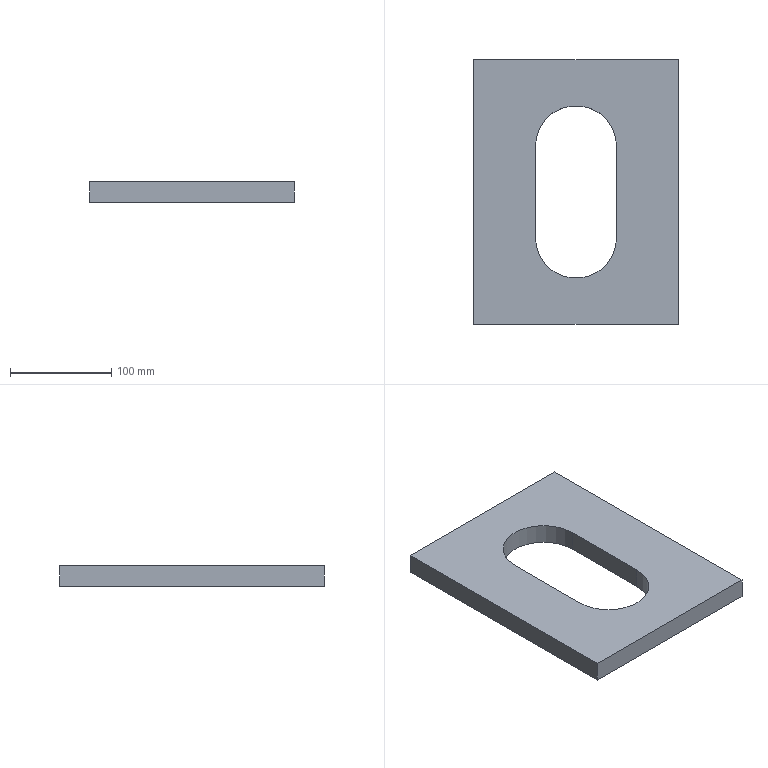Part | SolidWorks | features Cut 1, Extrusion 1 | 1 solid | 10 faces | box 202 x 261 x 20 mm | volume 809909 mm3 | plane 8 | cylinder 2 | commonest cylinder face diameters 80 x2
STEP:
#1=CARTESIAN_POINT('',(-75.,-256.,0.));
#2=VERTEX_POINT('',#1);
#3=CARTESIAN_POINT('',(-75.,5.,0.));
#4=VERTEX_POINT('',#3);
#5=CARTESIAN_POINT('',(-75.,5.,0.));
#6=DIRECTION('',(0.,1.,0.));
#7=VECTOR('',#6,1000.);
#8=LINE('',#5,#7);
#9=EDGE_CURVE('',#2,#4,#8,.T.);
#10=ORIENTED_EDGE('',*,*,#9,.T.);
#11=CARTESIAN_POINT('',(-75.,5.,20.));
#12=VERTEX_POINT('',#11);
#13=CARTESIAN_POINT('',(-75.,5.,20.));
#14=DIRECTION('',(0.,0.,-1.));
#15=VECTOR('',#14,1000.);
#16=LINE('',#13,#15);
#17=EDGE_CURVE('',#12,#4,#16,.T.);
#18=ORIENTED_EDGE('',*,*,#17,.F.);
#19=CARTESIAN_POINT('',(-75.,-256.,20.));
#20=VERTEX_POINT('',#19);
#21=CARTESIAN_POINT('',(-75.,5.,20.));
#22=DIRECTION('',(0.,1.,0.));
#23=VECTOR('',#22,1000.);
#24=LINE('',#21,#23);
#25=EDGE_CURVE('',#20,#12,#24,.T.);
#26=ORIENTED_EDGE('',*,*,#25,.F.);
#27=CARTESIAN_POINT('',(-75.,-256.,20.));
#28=DIRECTION('',(0.,0.,-1.));
#29=VECTOR('',#28,1000.);
#30=LINE('',#27,#29);
#31=EDGE_CURVE('',#20,#2,#30,.T.);
#32=ORIENTED_EDGE('',*,*,#31,.T.);
#33=EDGE_LOOP('',(#10,#18,#26,#32));
#34=FACE_OUTER_BOUND('',#33,.T.);
#35=CARTESIAN_POINT('',(-75.,5.,20.));
#36=DIRECTION('',(-1.,0.,0.));
#37=DIRECTION('',(0.,-1.,0.));
#38=AXIS2_PLACEMENT_3D('',#35,#36,#37);
#39=PLANE('',#38);
#40=ADVANCED_FACE('',(#34),#39,.F.);
#41=CARTESIAN_POINT('',(-277.,5.,0.));
#42=VERTEX_POINT('',#41);
#43=CARTESIAN_POINT('',(-75.,5.,0.));
#44=DIRECTION('',(-1.,0.,0.));
#45=VECTOR('',#44,1000.);
#46=LINE('',#43,#45);
#47=EDGE_CURVE('',#4,#42,#46,.T.);
#48=ORIENTED_EDGE('',*,*,#47,.T.);
#49=CARTESIAN_POINT('',(-277.,5.,20.));
#50=VERTEX_POINT('',#49);
#51=CARTESIAN_POINT('',(-277.,5.,20.));
#52=DIRECTION('',(0.,0.,-1.));
#53=VECTOR('',#52,1000.);
#54=LINE('',#51,#53);
#55=EDGE_CURVE('',#50,#42,#54,.T.);
#56=ORIENTED_EDGE('',*,*,#55,.F.);
#57=CARTESIAN_POINT('',(-75.,5.,20.));
#58=DIRECTION('',(-1.,0.,0.));
#59=VECTOR('',#58,1000.);
#60=LINE('',#57,#59);
#61=EDGE_CURVE('',#12,#50,#60,.T.);
#62=ORIENTED_EDGE('',*,*,#61,.F.);
#63=ORIENTED_EDGE('',*,*,#17,.T.);
#64=EDGE_LOOP('',(#48,#56,#62,#63));
#65=FACE_OUTER_BOUND('',#64,.T.);
#66=CARTESIAN_POINT('',(-75.,5.,20.));
#67=DIRECTION('',(0.,-1.,0.));
#68=DIRECTION('',(1.,0.,0.));
#69=AXIS2_PLACEMENT_3D('',#66,#67,#68);
#70=PLANE('',#69);
#71=ADVANCED_FACE('',(#65),#70,.F.);
#72=CARTESIAN_POINT('',(-277.,-256.,0.));
#73=VERTEX_POINT('',#72);
#74=CARTESIAN_POINT('',(-277.,5.,0.));
#75=DIRECTION('',(0.,-1.,0.));
#76=VECTOR('',#75,1000.);
#77=LINE('',#74,#76);
#78=EDGE_CURVE('',#42,#73,#77,.T.);
#79=ORIENTED_EDGE('',*,*,#78,.T.);
#80=CARTESIAN_POINT('',(-277.,-256.,20.));
#81=VERTEX_POINT('',#80);
#82=CARTESIAN_POINT('',(-277.,-256.,20.));
#83=DIRECTION('',(0.,0.,-1.));
#84=VECTOR('',#83,1000.);
#85=LINE('',#82,#84);
#86=EDGE_CURVE('',#81,#73,#85,.T.);
#87=ORIENTED_EDGE('',*,*,#86,.F.);
#88=CARTESIAN_POINT('',(-277.,5.,20.));
#89=DIRECTION('',(0.,-1.,0.));
#90=VECTOR('',#89,1000.);
#91=LINE('',#88,#90);
#92=EDGE_CURVE('',#50,#81,#91,.T.);
#93=ORIENTED_EDGE('',*,*,#92,.F.);
#94=ORIENTED_EDGE('',*,*,#55,.T.);
#95=EDGE_LOOP('',(#79,#87,#93,#94));
#96=FACE_OUTER_BOUND('',#95,.T.);
#97=CARTESIAN_POINT('',(-277.,5.,20.));
#98=DIRECTION('',(1.,0.,0.));
#99=DIRECTION('',(0.,0.,-1.));
#100=AXIS2_PLACEMENT_3D('',#97,#98,#99);
#101=PLANE('',#100);
#102=ADVANCED_FACE('',(#96),#101,.F.);
#103=CARTESIAN_POINT('',(-75.,-256.,0.));
#104=DIRECTION('',(1.,0.,0.));
#105=VECTOR('',#104,1000.);
#106=LINE('',#103,#105);
#107=EDGE_CURVE('',#73,#2,#106,.T.);
#108=ORIENTED_EDGE('',*,*,#107,.T.);
#109=ORIENTED_EDGE('',*,*,#31,.F.);
#110=CARTESIAN_POINT('',(-75.,-256.,20.));
#111=DIRECTION('',(1.,0.,0.));
#112=VECTOR('',#111,1000.);
#113=LINE('',#110,#112);
#114=EDGE_CURVE('',#81,#20,#113,.T.);
#115=ORIENTED_EDGE('',*,*,#114,.F.);
#116=ORIENTED_EDGE('',*,*,#86,.T.);
#117=EDGE_LOOP('',(#108,#109,#115,#116));
#118=FACE_OUTER_BOUND('',#117,.T.);
#119=CARTESIAN_POINT('',(-75.,-256.,20.));
#120=DIRECTION('',(0.,1.,0.));
#121=DIRECTION('',(0.,0.,1.));
#122=AXIS2_PLACEMENT_3D('',#119,#120,#121);
#123=PLANE('',#122);
#124=ADVANCED_FACE('',(#118),#123,.F.);
#125=CARTESIAN_POINT('',(-136.,-170.5,20.));
#126=VERTEX_POINT('',#125);
#127=CARTESIAN_POINT('',(-136.,-80.5,20.));
#128=VERTEX_POINT('',#127);
#129=CARTESIAN_POINT('',(-136.,-170.5,20.));
#130=DIRECTION('',(0.,1.,0.));
#131=VECTOR('',#130,1000.);
#132=LINE('',#129,#131);
#133=EDGE_CURVE('',#126,#128,#132,.T.);
#134=ORIENTED_EDGE('',*,*,#133,.F.);
#135=CARTESIAN_POINT('',(-216.,-170.5,20.));
#136=VERTEX_POINT('',#135);
#137=CARTESIAN_POINT('',(-176.,-170.5,20.));
#138=DIRECTION('',(0.,0.,1.));
#139=DIRECTION('',(1.,0.,0.));
#140=AXIS2_PLACEMENT_3D('',#137,#138,#139);
#141=CIRCLE('',#140,40.);
#142=EDGE_CURVE('',#136,#126,#141,.T.);
#143=ORIENTED_EDGE('',*,*,#142,.F.);
#144=CARTESIAN_POINT('',(-216.,-80.5,20.));
#145=VERTEX_POINT('',#144);
#146=CARTESIAN_POINT('',(-216.,-170.5,20.));
#147=DIRECTION('',(0.,-1.,0.));
#148=VECTOR('',#147,1000.);
#149=LINE('',#146,#148);
#150=EDGE_CURVE('',#145,#136,#149,.T.);
#151=ORIENTED_EDGE('',*,*,#150,.F.);
#152=CARTESIAN_POINT('',(-176.,-80.5,20.));
#153=DIRECTION('',(0.,0.,1.));
#154=DIRECTION('',(1.,0.,0.));
#155=AXIS2_PLACEMENT_3D('',#152,#153,#154);
#156=CIRCLE('',#155,40.);
#157=EDGE_CURVE('',#128,#145,#156,.T.);
#158=ORIENTED_EDGE('',*,*,#157,.F.);
#159=EDGE_LOOP('',(#134,#143,#151,#158));
#160=FACE_BOUND('',#159,.T.);
#161=ORIENTED_EDGE('',*,*,#25,.T.);
#162=ORIENTED_EDGE('',*,*,#61,.T.);
#163=ORIENTED_EDGE('',*,*,#92,.T.);
#164=ORIENTED_EDGE('',*,*,#114,.T.);
#165=EDGE_LOOP('',(#161,#162,#163,#164));
#166=FACE_OUTER_BOUND('',#165,.T.);
#167=CARTESIAN_POINT('',(0.,0.,20.));
#168=DIRECTION('',(0.,0.,-1.));
#169=DIRECTION('',(-1.,0.,0.));
#170=AXIS2_PLACEMENT_3D('',#167,#168,#169);
#171=PLANE('',#170);
#172=ADVANCED_FACE('',(#160,#166),#171,.F.);
#173=CARTESIAN_POINT('',(-216.,-170.5,0.));
#174=VERTEX_POINT('',#173);
#175=CARTESIAN_POINT('',(-136.,-170.5,0.));
#176=VERTEX_POINT('',#175);
#177=CARTESIAN_POINT('',(-176.,-170.5,0.));
#178=DIRECTION('',(0.,0.,1.));
#179=DIRECTION('',(1.,0.,0.));
#180=AXIS2_PLACEMENT_3D('',#177,#178,#179);
#181=CIRCLE('',#180,40.);
#182=EDGE_CURVE('',#174,#176,#181,.T.);
#183=ORIENTED_EDGE('',*,*,#182,.T.);
#184=CARTESIAN_POINT('',(-136.,-80.5,0.));
#185=VERTEX_POINT('',#184);
#186=CARTESIAN_POINT('',(-136.,-170.5,0.));
#187=DIRECTION('',(0.,1.,0.));
#188=VECTOR('',#187,1000.);
#189=LINE('',#186,#188);
#190=EDGE_CURVE('',#176,#185,#189,.T.);
#191=ORIENTED_EDGE('',*,*,#190,.T.);
#192=CARTESIAN_POINT('',(-216.,-80.5,0.));
#193=VERTEX_POINT('',#192);
#194=CARTESIAN_POINT('',(-176.,-80.5,0.));
#195=DIRECTION('',(0.,0.,1.));
#196=DIRECTION('',(1.,0.,0.));
#197=AXIS2_PLACEMENT_3D('',#194,#195,#196);
#198=CIRCLE('',#197,40.);
#199=EDGE_CURVE('',#185,#193,#198,.T.);
#200=ORIENTED_EDGE('',*,*,#199,.T.);
#201=CARTESIAN_POINT('',(-216.,-170.5,0.));
#202=DIRECTION('',(0.,-1.,0.));
#203=VECTOR('',#202,1000.);
#204=LINE('',#201,#203);
#205=EDGE_CURVE('',#193,#174,#204,.T.);
#206=ORIENTED_EDGE('',*,*,#205,.T.);
#207=EDGE_LOOP('',(#183,#191,#200,#206));
#208=FACE_BOUND('',#207,.T.);
#209=ORIENTED_EDGE('',*,*,#9,.F.);
#210=ORIENTED_EDGE('',*,*,#107,.F.);
#211=ORIENTED_EDGE('',*,*,#78,.F.);
#212=ORIENTED_EDGE('',*,*,#47,.F.);
#213=EDGE_LOOP('',(#209,#210,#211,#212));
#214=FACE_OUTER_BOUND('',#213,.T.);
#215=CARTESIAN_POINT('',(0.,0.,0.));
#216=DIRECTION('',(0.,0.,-1.));
#217=DIRECTION('',(-1.,0.,0.));
#218=AXIS2_PLACEMENT_3D('',#215,#216,#217);
#219=PLANE('',#218);
#220=ADVANCED_FACE('',(#208,#214),#219,.T.);
#221=ORIENTED_EDGE('',*,*,#142,.T.);
#222=CARTESIAN_POINT('',(-136.,-170.5,0.));
#223=DIRECTION('',(0.,0.,1.));
#224=VECTOR('',#223,1000.);
#225=LINE('',#222,#224);
#226=EDGE_CURVE('',#176,#126,#225,.T.);
#227=ORIENTED_EDGE('',*,*,#226,.F.);
#228=ORIENTED_EDGE('',*,*,#182,.F.);
#229=CARTESIAN_POINT('',(-216.,-170.5,0.));
#230=DIRECTION('',(0.,0.,1.));
#231=VECTOR('',#230,1000.);
#232=LINE('',#229,#231);
#233=EDGE_CURVE('',#174,#136,#232,.T.);
#234=ORIENTED_EDGE('',*,*,#233,.T.);
#235=EDGE_LOOP('',(#221,#227,#228,#234));
#236=FACE_OUTER_BOUND('',#235,.T.);
#237=CARTESIAN_POINT('',(-176.,-170.5,0.));
#238=DIRECTION('',(0.,0.,1.));
#239=DIRECTION('',(1.,0.,0.));
#240=AXIS2_PLACEMENT_3D('',#237,#238,#239);
#241=CYLINDRICAL_SURFACE('',#240,40.);
#242=ADVANCED_FACE('',(#236),#241,.F.);
#243=ORIENTED_EDGE('',*,*,#150,.T.);
#244=ORIENTED_EDGE('',*,*,#233,.F.);
#245=ORIENTED_EDGE('',*,*,#205,.F.);
#246=CARTESIAN_POINT('',(-216.,-80.5,0.));
#247=DIRECTION('',(0.,0.,1.));
#248=VECTOR('',#247,1000.);
#249=LINE('',#246,#248);
#250=EDGE_CURVE('',#193,#145,#249,.T.);
#251=ORIENTED_EDGE('',*,*,#250,.T.);
#252=EDGE_LOOP('',(#243,#244,#245,#251));
#253=FACE_OUTER_BOUND('',#252,.T.);
#254=CARTESIAN_POINT('',(-216.,-170.5,0.));
#255=DIRECTION('',(-1.,0.,0.));
#256=DIRECTION('',(0.,-1.,0.));
#257=AXIS2_PLACEMENT_3D('',#254,#255,#256);
#258=PLANE('',#257);
#259=ADVANCED_FACE('',(#253),#258,.F.);
#260=ORIENTED_EDGE('',*,*,#157,.T.);
#261=ORIENTED_EDGE('',*,*,#250,.F.);
#262=ORIENTED_EDGE('',*,*,#199,.F.);
#263=CARTESIAN_POINT('',(-136.,-80.5,0.));
#264=DIRECTION('',(0.,0.,1.));
#265=VECTOR('',#264,1000.);
#266=LINE('',#263,#265);
#267=EDGE_CURVE('',#185,#128,#266,.T.);
#268=ORIENTED_EDGE('',*,*,#267,.T.);
#269=EDGE_LOOP('',(#260,#261,#262,#268));
#270=FACE_OUTER_BOUND('',#269,.T.);
#271=CARTESIAN_POINT('',(-176.,-80.5,0.));
#272=DIRECTION('',(0.,0.,1.));
#273=DIRECTION('',(1.,0.,0.));
#274=AXIS2_PLACEMENT_3D('',#271,#272,#273);
#275=CYLINDRICAL_SURFACE('',#274,40.);
#276=ADVANCED_FACE('',(#270),#275,.F.);
#277=ORIENTED_EDGE('',*,*,#133,.T.);
#278=ORIENTED_EDGE('',*,*,#267,.F.);
#279=ORIENTED_EDGE('',*,*,#190,.F.);
#280=ORIENTED_EDGE('',*,*,#226,.T.);
#281=EDGE_LOOP('',(#277,#278,#279,#280));
#282=FACE_OUTER_BOUND('',#281,.T.);
#283=CARTESIAN_POINT('',(-136.,-170.5,0.));
#284=DIRECTION('',(1.,0.,0.));
#285=DIRECTION('',(0.,1.,0.));
#286=AXIS2_PLACEMENT_3D('',#283,#284,#285);
#287=PLANE('',#286);
#288=ADVANCED_FACE('',(#282),#287,.F.);
#289=CLOSED_SHELL('',(#40,#71,#102,#124,#172,#220,#242,#259,#276,#288));
#290=MANIFOLD_SOLID_BREP('',#289);
#291=CARTESIAN_POINT('',(0.,0.,0.));
#292=DIRECTION('',(0.,0.,1.));
#293=DIRECTION('',(1.,0.,0.));
#294=AXIS2_PLACEMENT_3D('',#291,#292,#293);
#295=(LENGTH_UNIT()NAMED_UNIT(*)SI_UNIT(.MILLI.,.METRE.));
#296=UNCERTAINTY_MEASURE_WITH_UNIT(LENGTH_MEASURE(0.00001),#295,'','');
#297=(NAMED_UNIT(*)PLANE_ANGLE_UNIT()SI_UNIT($,.RADIAN.));
#298=(NAMED_UNIT(*)SI_UNIT($,.STERADIAN.)SOLID_ANGLE_UNIT());
#299=(GEOMETRIC_REPRESENTATION_CONTEXT(3)GLOBAL_UNCERTAINTY_ASSIGNED_CONTEXT((#296))GLOBAL_UNIT_ASSIGNED_CONTEXT((#295,#297,#298))REPRESENTATION_CONTEXT('',''));
#300=ADVANCED_BREP_SHAPE_REPRESENTATION('',(#290,#294),#299);